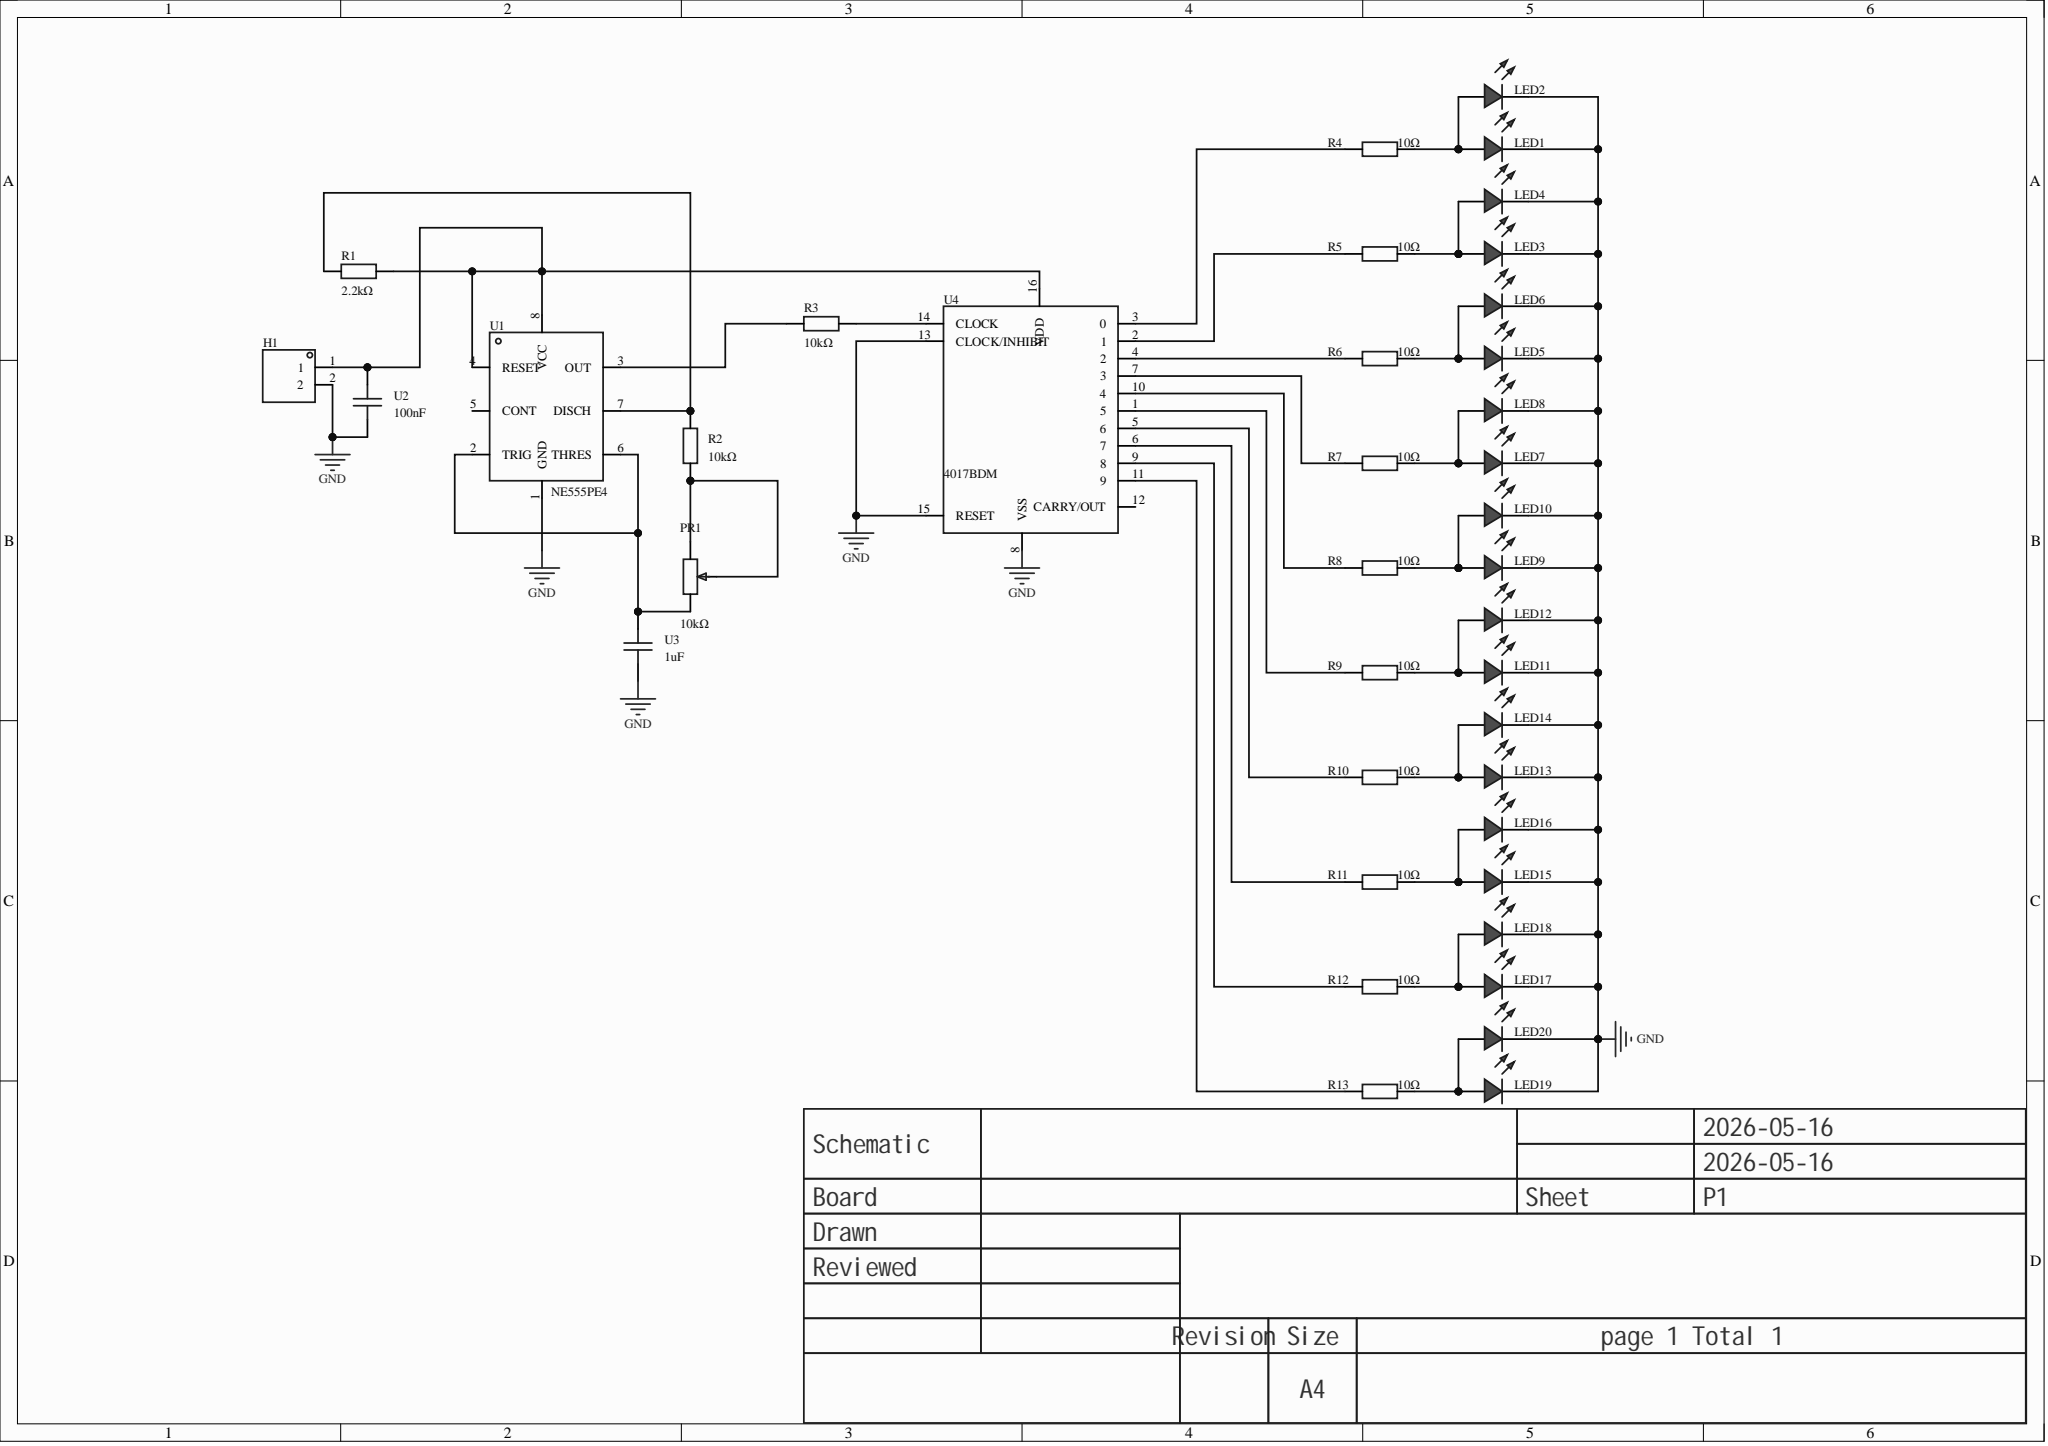Circuit board | Altium Designer | 39 parts | 27 nets
Bill of materials:
Comment,Description,Designator,Footprint,LibRef,Quantity
"","","H1","HDR-TH_2P-P2.54-V-M-1","HDR-M_2.54_1x2P","1"
"","","LED1, LED2, LED3, LED4, LED5, LED6, LED7, LED8, LED9, LED10, LED11, LED12, LED13, LED14, LED15, LED16, LED17, LED18, LED19, LED20","LED_TH-3mm","LED_TH-R_3mm","20"
"10kΩ","","PR1","R_3296","R_3296","1"
"2.2kΩ","","R1","Res_1/8W","Res_AXIAL-1/8W","1"
"10kΩ","","R2, R3","Res_1/8W","Res_AXIAL-1/8W","2"
"10Ω","","R4, R5, R6, R7, R8, R9, R10, R11, R12, R13","Res_1/8W","Res_AXIAL-1/8W","10"
"NE555PE4","NE555 single timer","U1","PDIP-8_L9.6-W6.4-P2.54-LS7.9-BL-1","NE555PE4","1"
"100nF","","U2","CAP-TH_L5.0-W2.5-P5.00-D1.0","100nF","1"
"1uF","","U3","CAP-TH_L5.0-W2.5-P5.00-D1.0","100nF","1"
"4017BDM","Operating voltage: 3V~15V; Number of components: 1; Bits per component: 5; Trigger type: positive edge; negative edge;","U4","PDIP-16_L19.3-W6.5-P2.54-LS7.6-BL","4017BDM","1"
Netlist (Protel format):
[
H1
HDR-TH_2P-P2.54-V-M-1




]
[
LED1
LED_TH-3mm




]
[
LED2
LED_TH-3mm




]
[
LED3
LED_TH-3mm




]
[
LED4
LED_TH-3mm




]
[
LED5
LED_TH-3mm




]
[
LED6
LED_TH-3mm




]
[
LED7
LED_TH-3mm




]
[
LED8
LED_TH-3mm




]
[
LED9
LED_TH-3mm




]
[
LED10
LED_TH-3mm




]
[
LED11
LED_TH-3mm




]
[
LED12
LED_TH-3mm




]
[
LED13
LED_TH-3mm




]
[
LED14
LED_TH-3mm




]
[
LED15
LED_TH-3mm




]
[
LED16
LED_TH-3mm




]
[
LED17
LED_TH-3mm




]
[
LED18
LED_TH-3mm




]
[
LED19
LED_TH-3mm




]
[
LED20
LED_TH-3mm




]
[
PR1
R_3296
10kΩ



]
[
R1
Res_1/8W
2.2kΩ



]
[
R2
Res_1/8W
10kΩ



]
[
R3
Res_1/8W
10kΩ



]
[
R4
Res_1/8W
10Ω



]
[
R5
Res_1/8W
10Ω



]
[
R6
Res_1/8W
10Ω



]
[
R7
Res_1/8W
10Ω



]
[
R8
Res_1/8W
10Ω



]
[
R9
Res_1/8W
10Ω



]
[
R10
Res_1/8W
10Ω



]
[
R11
Res_1/8W
10Ω



]
[
R12
Res_1/8W
10Ω



]
[
R13
Res_1/8W
10Ω



]
[
U1
PDIP-8_L9.6-W6.4-P2.54-LS7.9-BL-1
NE555PE4



]
[
U2
CAP-TH_L5.0-W2.5-P5.00-D1.0
100nF



]
[
U3
CAP-TH_L5.0-W2.5-P5.00-D1.0
1uF



]
[
U4
PDIP-16_L19.3-W6.5-P2.54-LS7.6-BL
4017BDM



]
(
NetR13_1
R13-1
U4-11
)
(
NetR12_1
R12-1
U4-9
)
(
NetR11_1
R11-1
U4-6
)
(
NetR10_1
R10-1
U4-5
)
(
NetR9_1
R9-1
U4-1
)
(
NetR8_1
R8-1
U4-10
)
(
NetR7_1
R7-1
U4-7
)
(
NetR6_1
R6-1
U4-4
)
(
NetR5_1
R5-1
U4-2
)
(
NetR4_1
R4-1
U4-3
)
(
NetR3_2
R3-2
U4-14
)
(
NetR3_1
R3-1
U1-3
)
(
NetR1_1
R1-1
R2-2
U1-7
)
(
NetPR1_2
PR1-2
PR1-3
R2-1
)
(
NetPR1_1
PR1-1
U1-2
U1-6
U3-1
)
(
NetLED19_1
LED19-1
LED20-1
R13-2
)
(
NetLED17_1
LED17-1
LED18-1
R12-2
)
(
NetLED15_1
LED15-1
LED16-1
R11-2
)
(
NetLED13_1
LED13-1
LED14-1
R10-2
)
(
NetLED11_1
LED11-1
LED12-1
R9-2
)
(
NetLED9_1
LED9-1
LED10-1
R8-2
)
(
NetLED7_1
LED7-1
LED8-1
R7-2
)
(
NetLED5_1
LED5-1
LED6-1
R6-2
)
(
NetLED3_1
LED3-1
LED4-1
R5-2
)
(
NetLED1_1
LED1-1
LED2-1
R4-2
)
(
NetH1_1
H1-1
R1-2
U1-4
U1-8
U2-1
U4-16
)
(
GND
H1-2
LED1-2
LED2-2
LED3-2
LED4-2
LED5-2
LED6-2
LED7-2
LED8-2
LED9-2
LED10-2
LED11-2
LED12-2
LED13-2
LED14-2
LED15-2
LED16-2
LED17-2
LED18-2
LED19-2
LED20-2
U1-1
U2-2
U3-2
U4-8
U4-13
U4-15
)